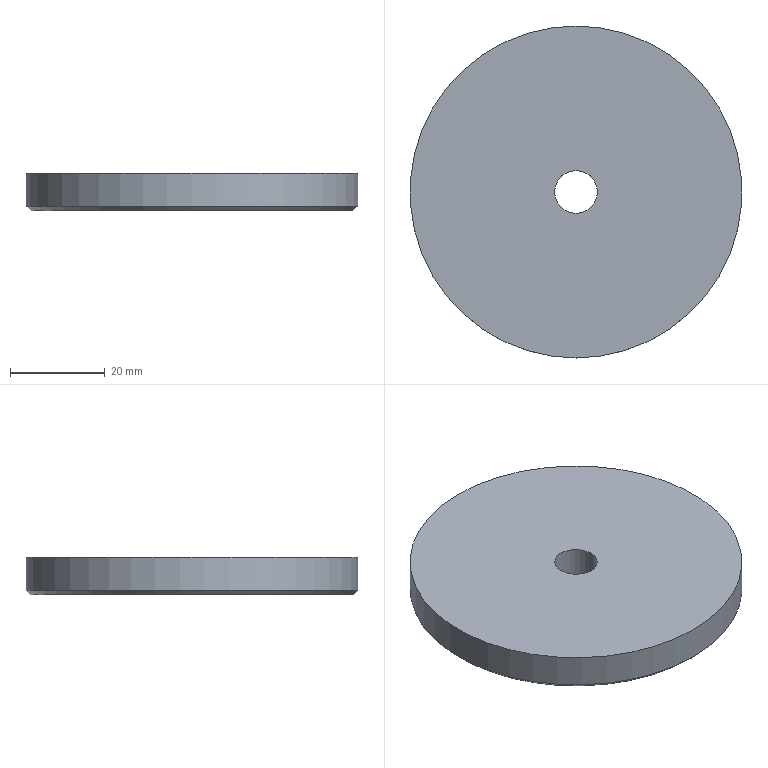Part | NX | features 11 2 | 1 solid | 5 faces | box 70 x 70 x 8 mm | volume 30170 mm3 | plane 2 | cylinder 2 | cone 1 | commonest cylinder face diameters 9 x1 70 x1
STEP:
#1=CARTESIAN_POINT('',(2985.,-566.5,159.));
#2=VERTEX_POINT('',#1);
#3=CARTESIAN_POINT('',(2985.,-600.5,159.));
#4=DIRECTION('',(0.,0.,-1.));
#5=DIRECTION('',(0.,1.,0.));
#6=AXIS2_PLACEMENT_3D('',#3,#4,#5);
#7=CIRCLE('',#6,34.);
#8=EDGE_CURVE('',#2,#2,#7,.T.);
#9=ORIENTED_EDGE('',*,*,#8,.T.);
#10=EDGE_LOOP('',(#9));
#11=FACE_BOUND('',#10,.T.);
#12=CARTESIAN_POINT('',(2985.,-596.,159.));
#13=VERTEX_POINT('',#12);
#14=CARTESIAN_POINT('',(2985.,-600.5,159.));
#15=DIRECTION('',(0.,0.,-1.));
#16=DIRECTION('',(0.,1.,0.));
#17=AXIS2_PLACEMENT_3D('',#14,#15,#16);
#18=CIRCLE('',#17,4.5);
#19=EDGE_CURVE('',#13,#13,#18,.T.);
#20=ORIENTED_EDGE('',*,*,#19,.F.);
#21=EDGE_LOOP('',(#20));
#22=FACE_BOUND('',#21,.T.);
#23=CARTESIAN_POINT('',(2985.,-600.5,159.));
#24=DIRECTION('',(0.,0.,1.));
#25=DIRECTION('',(0.,-1.,0.));
#26=AXIS2_PLACEMENT_3D('',#23,#24,#25);
#27=PLANE('',#26);
#28=ADVANCED_FACE('',(#11,#22),#27,.F.);
#29=CARTESIAN_POINT('',(2985.,-565.5,160.));
#30=VERTEX_POINT('',#29);
#31=CARTESIAN_POINT('',(2985.,-600.5,160.));
#32=DIRECTION('',(0.,0.,1.));
#33=DIRECTION('',(0.,1.,0.));
#34=AXIS2_PLACEMENT_3D('',#31,#32,#33);
#35=CIRCLE('',#34,35.);
#36=EDGE_CURVE('',#30,#30,#35,.T.);
#37=ORIENTED_EDGE('',*,*,#36,.T.);
#38=EDGE_LOOP('',(#37));
#39=FACE_BOUND('',#38,.T.);
#40=CARTESIAN_POINT('',(2985.,-565.5,167.));
#41=VERTEX_POINT('',#40);
#42=CARTESIAN_POINT('',(2985.,-600.5,167.));
#43=DIRECTION('',(0.,0.,1.));
#44=DIRECTION('',(0.,1.,0.));
#45=AXIS2_PLACEMENT_3D('',#42,#43,#44);
#46=CIRCLE('',#45,35.);
#47=EDGE_CURVE('',#41,#41,#46,.T.);
#48=ORIENTED_EDGE('',*,*,#47,.F.);
#49=EDGE_LOOP('',(#48));
#50=FACE_BOUND('',#49,.T.);
#51=CARTESIAN_POINT('',(2985.,-600.5,161.));
#52=DIRECTION('',(0.,0.,1.));
#53=DIRECTION('',(0.,-1.,0.));
#54=AXIS2_PLACEMENT_3D('',#51,#52,#53);
#55=CYLINDRICAL_SURFACE('',#54,35.);
#56=ADVANCED_FACE('',(#39,#50),#55,.T.);
#57=CARTESIAN_POINT('',(2985.,-596.,167.));
#58=VERTEX_POINT('',#57);
#59=CARTESIAN_POINT('',(2985.,-600.5,167.));
#60=DIRECTION('',(0.,0.,1.));
#61=DIRECTION('',(0.,1.,0.));
#62=AXIS2_PLACEMENT_3D('',#59,#60,#61);
#63=CIRCLE('',#62,4.5);
#64=EDGE_CURVE('',#58,#58,#63,.T.);
#65=ORIENTED_EDGE('',*,*,#64,.F.);
#66=EDGE_LOOP('',(#65));
#67=FACE_BOUND('',#66,.T.);
#68=ORIENTED_EDGE('',*,*,#47,.T.);
#69=EDGE_LOOP('',(#68));
#70=FACE_BOUND('',#69,.T.);
#71=CARTESIAN_POINT('',(2985.,-600.5,167.));
#72=DIRECTION('',(0.,0.,1.));
#73=DIRECTION('',(0.,-1.,0.));
#74=AXIS2_PLACEMENT_3D('',#71,#72,#73);
#75=PLANE('',#74);
#76=ADVANCED_FACE('',(#67,#70),#75,.T.);
#77=ORIENTED_EDGE('',*,*,#8,.F.);
#78=EDGE_LOOP('',(#77));
#79=FACE_BOUND('',#78,.T.);
#80=ORIENTED_EDGE('',*,*,#36,.F.);
#81=EDGE_LOOP('',(#80));
#82=FACE_BOUND('',#81,.T.);
#83=CARTESIAN_POINT('',(2985.,-600.5,160.));
#84=DIRECTION('',(0.,0.,1.));
#85=DIRECTION('',(0.,-1.,0.));
#86=AXIS2_PLACEMENT_3D('',#83,#84,#85);
#87=CONICAL_SURFACE('',#86,35.,0.7854);
#88=ADVANCED_FACE('',(#79,#82),#87,.T.);
#89=ORIENTED_EDGE('',*,*,#19,.T.);
#90=EDGE_LOOP('',(#89));
#91=FACE_BOUND('',#90,.T.);
#92=ORIENTED_EDGE('',*,*,#64,.T.);
#93=EDGE_LOOP('',(#92));
#94=FACE_BOUND('',#93,.T.);
#95=CARTESIAN_POINT('',(2985.,-600.5,161.));
#96=DIRECTION('',(0.,0.,1.));
#97=DIRECTION('',(0.,-1.,0.));
#98=AXIS2_PLACEMENT_3D('',#95,#96,#97);
#99=CYLINDRICAL_SURFACE('',#98,4.5);
#100=ADVANCED_FACE('',(#91,#94),#99,.F.);
#101=CLOSED_SHELL('',(#28,#56,#76,#88,#100));
#102=MANIFOLD_SOLID_BREP('',#101);
#103=(LENGTH_UNIT()NAMED_UNIT(*)SI_UNIT(.MILLI.,.METRE.));
#104=UNCERTAINTY_MEASURE_WITH_UNIT(LENGTH_MEASURE(0.00001),#103,'','');
#105=(NAMED_UNIT(*)PLANE_ANGLE_UNIT()SI_UNIT($,.RADIAN.));
#106=(NAMED_UNIT(*)SI_UNIT($,.STERADIAN.)SOLID_ANGLE_UNIT());
#107=(GEOMETRIC_REPRESENTATION_CONTEXT(3)GLOBAL_UNCERTAINTY_ASSIGNED_CONTEXT((#104))GLOBAL_UNIT_ASSIGNED_CONTEXT((#103,#105,#106))REPRESENTATION_CONTEXT('',''));
#108=ADVANCED_BREP_SHAPE_REPRESENTATION('',(#102),#107);